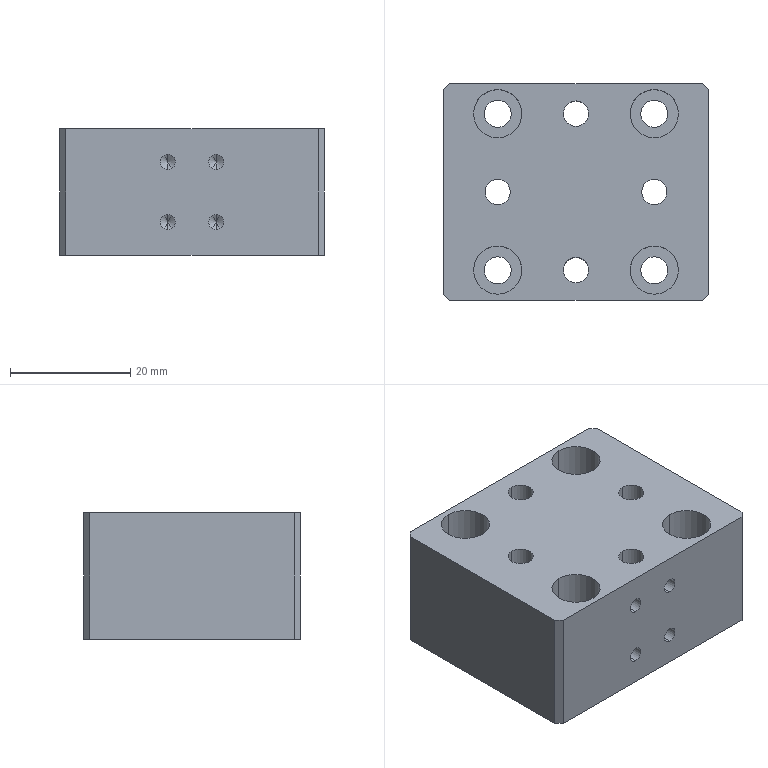NC program | NX | posted with a generic post | part box 44 x 36 x 21 mm
Whole program:
N10 G17 G21 G94 G90
(FLOOR_WALL , TOOL : D63)
N12 T01 M6
N14 G54
N16 G17 G0 G90 X-60.5 Y0. B0. C0. S6500 M3
N18 G43 Z30. H1
N20 Z3.
N22 G94 G1 Z0. F1250.
N24 X-57.5
N26 X57.5
N28 X60.5
N30 Z3.
N32 G0 Z30.
N34 M5
(DRILLING_COPY_1 , TOOL : D6A45)
N36 T07 M6
N38 G54
N40 G17 G0 G90 X-13. Y0. B0. C0. S5000 M3
N42 G43 Z30. H7
N44 G94 G81 G98 Z-2.6 F250. R3.
N46 Y13.
N48 X0.
N50 X13.
N52 Y0.
N54 Y-13.
N56 X0.
N58 X-13.
N60 G80
N62 G0 X-13. Y-13. Z30.
N64 M5
(DRILLING_COPY , TOOL : 4.2ZT)
N66 T14 M6
N68 G54
N70 G17 G0 G90 X-13. Y0. B0. C0. S2000 M3
N72 G43 Z30. H14
N74 G94 G83 G98 Z-23.762 F150. Q2. R3.
N76 X0. Y13.
N78 X13. Y0.
N80 X0. Y-13.
N82 G80
N84 G0 X0. Y-13. Z30.
N86 M5
(DRILLING_COPY_COPY_1 , TOOL : 4.5ZT)
N88 T16 M6
N90 G54
N92 G17 G0 G90 X-13. Y13. B0. C0. S2000 M3
N94 G43 Z30. H16
N96 G94 G83 G98 Z-23.852 F150. Q2. R3.
N98 X13.
N100 Y-13.
N102 X-13.
N104 G80
N106 G0 X-13. Y-13. Z30.
N108 M5
(HOLE_MILLING , TOOL : D4)
N110 T04 M6
N112 G54
N114 G17 G0 G90 X-13. Y13. B0. C0. S9500 M3
N116 G43 Z30. H4
N118 Z0.5
N120 G94 G3 X-12.01 Y12.01 R0.99 F1400.
N122 X-11.02 Y13. R0.99
N124 X-11.02 Y13. Z0. I-1.98 J0.
N126 X-11.02 Y13. Z-0.5 I-1.98 J0.
N128 X-11.02 Y13. Z-1. I-1.98 J0.
N130 X-11.02 Y13. Z-1.5 I-1.98 J0.
N132 X-11.02 Y13. Z-2. I-1.98 J0.
N134 X-11.02 Y13. Z-2.5 I-1.98 J0.
N136 X-11.02 Y13. Z-3. I-1.98 J0.
N138 X-11.02 Y13. Z-3.5 I-1.98 J0.
N140 X-11.02 Y13. Z-4. I-1.98 J0.
N142 X-11.02 Y13. Z-4.5 I-1.98 J0.
N144 X-11.02 Y13. Z-5. I-1.98 J0.
N146 X-11.02 Y13. Z-5.5 I-1.98 J0.
N148 X-11.02 Y13. Z-6. I-1.98 J0.
N150 X-11.02 Y13. Z-6.5 I-1.98 J0.
N152 X-11.02 Y13. Z-7. I-1.98 J0.
N154 X-11.02 Y13. Z-7.5 I-1.98 J0.
N156 X-11.02 Y13. Z-8. I-1.98 J0.
N158 X-11.02 Y13. Z-8.5 I-1.98 J0.
N160 X-11.02 Y13. Z-9. I-1.98 J0.
N162 X-11.02 Y13. Z-9.5 I-1.98 J0.
N164 X-11.02 Y13. Z-10. I-1.98 J0.
N166 X-11.02 Y13. Z-10.5 I-1.98 J0.
N168 X-11.02 Y13. Z-11. I-1.98 J0.
N170 X-11.02 Y13. Z-11.5 I-1.98 J0.
N172 X-11.02 Y13. Z-12. I-1.98 J0.
N174 X-11.02 Y13. Z-12.5 I-1.98 J0.
N176 X-11.02 Y13. Z-13. I-1.98 J0.
N178 X-11.02 Y13. Z-13.5 I-1.98 J0.
N180 X-11.02 Y13. Z-14. I-1.98 J0.
N182 X-11.02 Y13. Z-14.5 I-1.98 J0.
N184 X-11.02 Y13. Z-15. I-1.98 J0.
N186 X-13. Y14.98 R1.98
N188 X-11.02 Y13. R-1.98
N190 X-12.01 Y13.99 R0.99
N192 X-13. Y13. R0.99
N194 G0 Z30.
N196 X13.
N198 Z0.5
N200 G3 X13.99 Y12.01 R0.99
N202 X14.98 Y13. R0.99
N204 X14.98 Y13. Z0. I-1.98 J0.
N206 X14.98 Y13. Z-0.5 I-1.98 J0.
N208 X14.98 Y13. Z-1. I-1.98 J0.
N210 X14.98 Y13. Z-1.5 I-1.98 J0.
N212 X14.98 Y13. Z-2. I-1.98 J0.
N214 X14.98 Y13. Z-2.5 I-1.98 J0.
N216 X14.98 Y13. Z-3. I-1.98 J0.
N218 X14.98 Y13. Z-3.5 I-1.98 J0.
N220 X14.98 Y13. Z-4. I-1.98 J0.
N222 X14.98 Y13. Z-4.5 I-1.98 J0.
N224 X14.98 Y13. Z-5. I-1.98 J0.
N226 X14.98 Y13. Z-5.5 I-1.98 J0.
N228 X14.98 Y13. Z-6. I-1.98 J0.
N230 X14.98 Y13. Z-6.5 I-1.98 J0.
N232 X14.98 Y13. Z-7. I-1.98 J0.
N234 X14.98 Y13. Z-7.5 I-1.98 J0.
N236 X14.98 Y13. Z-8. I-1.98 J0.
N238 X14.98 Y13. Z-8.5 I-1.98 J0.
N240 X14.98 Y13. Z-9. I-1.98 J0.
N242 X14.98 Y13. Z-9.5 I-1.98 J0.
N244 X14.98 Y13. Z-10. I-1.98 J0.
N246 X14.98 Y13. Z-10.5 I-1.98 J0.
N248 X14.98 Y13. Z-11. I-1.98 J0.
N250 X14.98 Y13. Z-11.5 I-1.98 J0.
N252 X14.98 Y13. Z-12. I-1.98 J0.
N254 X14.98 Y13. Z-12.5 I-1.98 J0.
N256 X14.98 Y13. Z-13. I-1.98 J0.
N258 X14.98 Y13. Z-13.5 I-1.98 J0.
N260 X14.98 Y13. Z-14. I-1.98 J0.
N262 X14.98 Y13. Z-14.5 I-1.98 J0.
N264 X14.98 Y13. Z-15. I-1.98 J0.
N266 X13. Y14.98 R1.98
N268 X14.98 Y13. R-1.98
N270 X13.99 Y13.99 R0.99
N272 X13. Y13. R0.99
N274 G0 Z30.
N276 Y-13.
N278 Z0.5
N280 G3 X13.99 Y-13.99 R0.99
N282 X14.98 Y-13. R0.99
N284 X14.98 Y-13. Z0. I-1.98 J0.
N286 X14.98 Y-13. Z-0.5 I-1.98 J0.
N288 X14.98 Y-13. Z-1. I-1.98 J0.
N290 X14.98 Y-13. Z-1.5 I-1.98 J0.
N292 X14.98 Y-13. Z-2. I-1.98 J0.
N294 X14.98 Y-13. Z-2.5 I-1.98 J0.
N296 X14.98 Y-13. Z-3. I-1.98 J0.
N298 X14.98 Y-13. Z-3.5 I-1.98 J0.
N300 X14.98 Y-13. Z-4. I-1.98 J0.
N302 X14.98 Y-13. Z-4.5 I-1.98 J0.
N304 X14.98 Y-13. Z-5. I-1.98 J0.
N306 X14.98 Y-13. Z-5.5 I-1.98 J0.
N308 X14.98 Y-13. Z-6. I-1.98 J0.
N310 X14.98 Y-13. Z-6.5 I-1.98 J0.
N312 X14.98 Y-13. Z-7. I-1.98 J0.
N314 X14.98 Y-13. Z-7.5 I-1.98 J0.
N316 X14.98 Y-13. Z-8. I-1.98 J0.
N318 X14.98 Y-13. Z-8.5 I-1.98 J0.
N320 X14.98 Y-13. Z-9. I-1.98 J0.
N322 X14.98 Y-13. Z-9.5 I-1.98 J0.
N324 X14.98 Y-13. Z-10. I-1.98 J0.
N326 X14.98 Y-13. Z-10.5 I-1.98 J0.
N328 X14.98 Y-13. Z-11. I-1.98 J0.
N330 X14.98 Y-13. Z-11.5 I-1.98 J0.
N332 X14.98 Y-13. Z-12. I-1.98 J0.
N334 X14.98 Y-13. Z-12.5 I-1.98 J0.
N336 X14.98 Y-13. Z-13. I-1.98 J0.
N338 X14.98 Y-13. Z-13.5 I-1.98 J0.
N340 X14.98 Y-13. Z-14. I-1.98 J0.
N342 X14.98 Y-13. Z-14.5 I-1.98 J0.
N344 X14.98 Y-13. Z-15. I-1.98 J0.
N346 X13. Y-11.02 R1.98
N348 X14.98 Y-13. R-1.98
N350 X13.99 Y-12.01 R0.99
N352 X13. Y-13. R0.99
N354 G0 Z30.
N356 X-13.
N358 Z0.5
N360 G3 X-12.01 Y-13.99 R0.99
N362 X-11.02 Y-13. R0.99
N364 X-11.02 Y-13. Z0. I-1.98 J0.
N366 X-11.02 Y-13. Z-0.5 I-1.98 J0.
N368 X-11.02 Y-13. Z-1. I-1.98 J0.
N370 X-11.02 Y-13. Z-1.5 I-1.98 J0.
N372 X-11.02 Y-13. Z-2. I-1.98 J0.
N374 X-11.02 Y-13. Z-2.5 I-1.98 J0.
N376 X-11.02 Y-13. Z-3. I-1.98 J0.
N378 X-11.02 Y-13. Z-3.5 I-1.98 J0.
N380 X-11.02 Y-13. Z-4. I-1.98 J0.
N382 X-11.02 Y-13. Z-4.5 I-1.98 J0.
N384 X-11.02 Y-13. Z-5. I-1.98 J0.
N386 X-11.02 Y-13. Z-5.5 I-1.98 J0.
N388 X-11.02 Y-13. Z-6. I-1.98 J0.
N390 X-11.02 Y-13. Z-6.5 I-1.98 J0.
N392 X-11.02 Y-13. Z-7. I-1.98 J0.
N394 X-11.02 Y-13. Z-7.5 I-1.98 J0.
N396 X-11.02 Y-13. Z-8. I-1.98 J0.
N398 X-11.02 Y-13. Z-8.5 I-1.98 J0.
N400 X-11.02 Y-13. Z-9. I-1.98 J0.
N402 X-11.02 Y-13. Z-9.5 I-1.98 J0.
N404 X-11.02 Y-13. Z-10. I-1.98 J0.
N406 X-11.02 Y-13. Z-10.5 I-1.98 J0.
N408 X-11.02 Y-13. Z-11. I-1.98 J0.
N410 X-11.02 Y-13. Z-11.5 I-1.98 J0.
N412 X-11.02 Y-13. Z-12. I-1.98 J0.
N414 X-11.02 Y-13. Z-12.5 I-1.98 J0.
N416 X-11.02 Y-13. Z-13. I-1.98 J0.
N418 X-11.02 Y-13. Z-13.5 I-1.98 J0.
N420 X-11.02 Y-13. Z-14. I-1.98 J0.
N422 X-11.02 Y-13. Z-14.5 I-1.98 J0.
N424 X-11.02 Y-13. Z-15. I-1.98 J0.
N426 X-13. Y-11.02 R1.98
N428 X-11.02 Y-13. R-1.98
N430 X-12.01 Y-12.01 R0.99
N432 X-13. Y-13. R0.99
N434 G0 Z30.
(HOLE_MILLING_COPY , TOOL : D4)
N436 Y13.
N438 Z0.5
N440 G3 X-12. Y12. R1.
N442 X-11. Y13. R1.
N444 X-11. Y13. Z-1.5 I-2. J0.
N446 X-11. Y13. Z-3.5 I-2. J0.
N448 X-11. Y13. Z-5.5 I-2. J0.
N450 X-11. Y13. Z-7.5 I-2. J0.
N452 X-11. Y13. Z-9.5 I-2. J0.
N454 X-11. Y13. Z-11.5 I-2. J0.
N456 X-11. Y13. Z-13.5 I-2. J0.
N458 X-13. Y11. Z-15. R-2.
N460 X-11. Y13. R2.
N462 X-13. Y11. R-2.
N464 X-12. Y12. R1.
N466 X-13. Y13. R1.
N468 G0 Z30.
N470 X13.
N472 Z0.5
N474 G3 X14. Y12. R1.
N476 X15. Y13. R1.
N478 X15. Y13. Z-1.5 I-2. J0.
N480 X15. Y13. Z-3.5 I-2. J0.
N482 X15. Y13. Z-5.5 I-2. J0.
N484 X15. Y13. Z-7.5 I-2. J0.
N486 X15. Y13. Z-9.5 I-2. J0.
N488 X15. Y13. Z-11.5 I-2. J0.
N490 X15. Y13. Z-13.5 I-2. J0.
N492 X13. Y11. Z-15. R-2.
N494 X15. Y13. R2.
N496 X13. Y11. R-2.
N498 X14. Y12. R1.
N500 X13. Y13. R1.
N502 G0 Z30.
N504 Y-13.
N506 Z0.5
N508 G3 X14. Y-14. R1.
N510 X15. Y-13. R1.
N512 X15. Y-13. Z-1.5 I-2. J0.
N514 X15. Y-13. Z-3.5 I-2. J0.
N516 X15. Y-13. Z-5.5 I-2. J0.
N518 X15. Y-13. Z-7.5 I-2. J0.
N520 X15. Y-13. Z-9.5 I-2. J0.
N522 X15. Y-13. Z-11.5 I-2. J0.
N524 X15. Y-13. Z-13.5 I-2. J0.
N526 X13. Y-15. Z-15. R-2.
N528 X15. Y-13. R2.
N530 X13. Y-15. R-2.
N532 X14. Y-14. R1.
N534 X13. Y-13. R1.
N536 G0 Z30.
N538 X-13.
N540 Z0.5
N542 G3 X-12. Y-14. R1.
N544 X-11. Y-13. R1.
N546 X-11. Y-13. Z-1.5 I-2. J0.
N548 X-11. Y-13. Z-3.5 I-2. J0.
N550 X-11. Y-13. Z-5.5 I-2. J0.
N552 X-11. Y-13. Z-7.5 I-2. J0.
N554 X-11. Y-13. Z-9.5 I-2. J0.
N556 X-11. Y-13. Z-11.5 I-2. J0.
N558 X-11. Y-13. Z-13.5 I-2. J0.
N560 X-13. Y-15. Z-15. R-2.
N562 X-11. Y-13. R2.
N564 X-13. Y-15. R-2.
N566 X-12. Y-14. R1.
N568 X-13. Y-13. R1.
N570 G0 Z30.
N572 M5
(ADAPTIVE_MILLING , TOOL : D10)
N574 T10 M6
N576 G54
N578 G17 G0 G90 X-33.697 Y-0.05 B0. C0. S9500 M3
N580 G43 Z30. H10
N582 Z-20.
N584 G94 G1 Z-21. F1000.
N586 X-32.34 Y-0.58 F3000.
N588 G3 X-31.05 Y-0.05 R1.015
N590 X-30.406 Y3.11 R9.424
N592 X-30.21 Y14.606 R185.073
N594 G2 X-30.164 Y19.904 R87.231
N596 X-27.107 Y24.146 R6.172
N598 X-21.408 Y25.863 R13.799
N600 X-11.818 Y26.181 R97.285
N602 G1 X-9.818 Y26.186
N604 X-6.418 Y26.189
N606 X4.482 Y26.19
N608 X23.282
N610 X23.382 Y26.189
N612 X23.482 Y26.186
N614 G2 X27.916 Y23.446 R5.892
N616 X29.812 Y17.813 R12.753
N618 X30.178 Y8.626 R81.53
N620 G1 X30.184 Y6.926
N622 X30.188 Y4.426
N624 X30.19 Y-0.574
N626 X30.191 Y-19.274
N628 X30.19 Y-19.374
N630 X30.187 Y-19.474
N632 G2 X27.452 Y-23.911 R5.888
N634 X21.821 Y-25.812 R12.766
N636 X13.133 Y-26.175 R76.729
N638 G1 X11.633 Y-26.182
N640 X9.533 Y-26.187
N642 X6.033 Y-26.189
N644 X-6.567 Y-26.19
N646 X-23.267
N648 X-23.367
N650 G2 X-27.732 Y-23.703 R5.738
N652 X-29.742 Y-18.325 R11.924
N654 X-30.171 Y-9.843 R63.748
N656 X-30.136 Y-2.144 R153.414
N658 G3 X-29.43 Y12.529 R119.594
N660 G2 X-29.366 Y17.427 R77.262
N662 X-25.308 Y23.173 R7.786
N664 X-19.116 Y24.995 R16.033
N666 X-9.728 Y25.365 R90.974
N668 G1 X-8.228 Y25.372
N670 X-6.128 Y25.377
N672 X-2.828 Y25.38
N674 X5.672 Y25.382
N676 X20.472
N678 X20.672 Y25.38
N680 G2 X26.938 Y21.67 R7.557
N682 X28.965 Y15.341 R15.177
N684 X29.361 Y6.455 R81.33
N686 G1 X29.369 Y5.055
N688 X29.375 Y3.355
N690 X29.379 Y0.755
N692 X29.382 Y-4.045
N694 Y-16.545
N696 X29.381 Y-16.645
N698 G2 X25.691 Y-22.923 R7.563
N700 X19.466 Y-24.95 R15.025
N702 X9.781 Y-25.364 R84.712
N704 G1 X8.281 Y-25.371
N706 X6.281 Y-25.376
N708 X3.081 Y-25.38
N710 X-4.219 Y-25.382
N712 X-20.519
N714 X-20.619 Y-25.381
N716 G2 X-26.964 Y-21.629 R7.577
N718 X-28.974 Y-15.295 R15.341
N720 X-29.03 Y0.681 R86.884
N722 G3 X-28.624 Y14.672 R206.127
N724 G2 X-23.838 Y22.258 R8.821
N726 X-21.472 Y23.305 R8.031
N728 X-13.975 Y24.417 R29.802
N730 X0.523 Y24.572 R399.715
N732 G1 X9.523 Y24.573
N734 X18.223
N736 X18.423 Y24.57
N738 X18.623 Y24.566
N740 X18.823 Y24.558
N742 X18.923 Y24.553
N744 G2 X26.171 Y19.952 R8.759
N746 X27.179 Y17.851 R6.56
N748 X28.387 Y10.574 R27.305
N750 X28.571 Y-3.323 R311.808
N752 X28.533 Y-15.222 R436.293
N754 X23.946 Y-22.176 R8.77
N756 X21.851 Y-23.179 R6.583
N758 X14.774 Y-24.371 R26.639
N760 X2.077 Y-24.57 R260.792
N762 G1 X-2.323 Y-24.572
N764 X-18.123 Y-24.573
N766 X-18.323 Y-24.572
N768 X-18.623 Y-24.566
N770 X-18.823 Y-24.558
N772 X-18.923 Y-24.553
N774 G2 X-26.183 Y-19.936 R8.78
N776 X-27.18 Y-17.852 R6.64
N778 X-28.392 Y-10.475 R27.444
N780 X-28.184 Y1.215 R92.775
N782 G3 X-27.833 Y13.008 R314.175
N784 G2 X-27.154 Y16.428 R13.151
N786 X-26.418 Y19.63 R6.131
N788 X-23.821 Y22.271 R10.862
N790 G1 X-23.63 Y22.418
N792 X-23.511 Y22.486
N794 G2 X-20.466 Y23.16 R6.28
N796 X-1.882 Y23.758 R211.897
N798 G1 X1.418 Y23.762
N800 X7.518 Y23.764
N802 X16.018 Y23.765
N804 X16.318 Y23.762
N806 X16.718 Y23.755
N808 X16.918 Y23.748
N810 G2 X20.28 Y23.15 R13.765
N812 X23.511 Y22.486 R6.269
N814 X26.21 Y19.9 R10.464
N816 G3 X27.903 Y20.947 R1.
N818 G1 X27.05 Y22.756 Z-20.9
N820 X26.408 Y24.119
N822 X26.318 Y24.266
N824 X26.21 Y24.4
N826 X25.587 Y25.007
N828 G3 X24.728 Y25.465 R2.608
N830 X21.706 Y26.16 R16.644
N832 X16.12 Y26.725 R75.358
N834 G1 X14.874 Y26.774
N836 X13.627 Y26.802
N838 X-18.516 Y27.047
N840 G3 X-19.169 Y26.811 R1.032
N842 G1 X-20.522 Y25.666
N844 X-21.034 Y25.24 Z-20.933
N846 X-21.529 Y24.795 Z-20.967
N848 G3 X-21.765 Y24.184 Z-21. R1.04
N850 X-20.766 Y23.15 R1.004
N852 G1 X20.334
N854 G2 X23.63 Y22.418 R6.139
N856 X26.486 Y19.511 R10.886
N858 X27.16 Y16.466 R6.28
N860 X27.752 Y0.082 R184.971
N862 X27.728 Y-13.317 R641.242
N864 X27.15 Y-16.278 R14.406
N866 X26.486 Y-19.511 R6.27
N868 X23.9 Y-22.21 R10.464
N870 G3 X24.947 Y-23.903 R1.
N872 G1 X26.756 Y-23.05 Z-20.9
N874 X28.119 Y-22.408
N876 X28.266 Y-22.318
N878 X28.4 Y-22.21
N880 X29.007 Y-21.587
N882 G3 X29.466 Y-20.728 R2.611
N884 X30.158 Y-17.706 R16.322
N886 X30.713 Y-12.12 R79.161
N888 G1 X30.763 Y-10.874
N890 X30.794 Y-9.628
N892 X31.047 Y14.516
N894 G3 X30.81 Y15.172 R1.032
N896 G1 X29.666 Y16.523
N898 X29.239 Y17.034 Z-20.933
N900 X28.795 Y17.53 Z-20.967
N902 G3 X28.183 Y17.765 Z-21. R1.04
N904 X27.15 Y16.766 R1.004
N906 G1 Y-16.334
N908 G2 X26.418 Y-19.63 R6.139
N910 X23.511 Y-22.486 R10.886
N912 X20.466 Y-23.16 R6.28
N914 X3.882 Y-23.752 R190.383
N916 G1 X1.582 Y-23.758
N918 X-1.718 Y-23.762
N920 X-8.318 Y-23.764
N922 X-16.018 Y-23.765
N924 X-16.318 Y-23.762
N926 X-16.718 Y-23.755
N928 G2 X-20.278 Y-23.15 R13.593
N930 X-23.511 Y-22.486 R6.271
N932 X-26.21 Y-19.9 R10.464
N934 G3 X-27.903 Y-20.947 R1.
N936 G1 X-27.05 Y-22.756 Z-20.9
N938 X-26.408 Y-24.119
N940 X-26.318 Y-24.266
N942 X-26.21 Y-24.4
N944 X-25.587 Y-25.007
N946 G3 X-24.728 Y-25.465 R2.608
N948 X-21.706 Y-26.16 R16.644
N950 X-16.12 Y-26.725 R75.358
N952 G1 X-14.874 Y-26.774
N954 X-13.627 Y-26.802
N956 X18.516 Y-27.047
N958 G3 X19.169 Y-26.811 R1.032
N960 G1 X20.522 Y-25.666
N962 X21.034 Y-25.24 Z-20.933
N964 X21.529 Y-24.795 Z-20.967
N966 G3 X21.765 Y-24.184 Z-21. R1.04
N968 X20.766 Y-23.15 R1.004
N970 G1 X-20.334
N972 G2 X-23.63 Y-22.418 R6.139
N974 X-26.486 Y-19.511 R10.886
N976 X-27.156 Y-16.566 R6.158
N978 X-27.658 Y-6.481 R153.028
N980 X-27.207 Y5.41 R516.415
N982 G3 X-27.15 Y16.522 R389.897
N984 X-28.252 Y17.62 R1.1
N986 X-29.35 Y16.522 R1.1
N988 G1 Y-16.766
N990 G3 X-28.248 Y-17.864 R1.1
N992 X-27.15 Y-16.766 R1.1
N994 G1 Y7.634
N996 G3 X-28.011 Y8.633 R1.016
N998 G1 X-29.604 Y8.871
N1000 Z-18.
N1002 G0 Z30.
N1004 M5
(ZLEVEL_PROFILE_COPY_COPY_1 , TOOL : D10JING)
N1006 T11 M6
N1008 G54
N1010 G17 G0 G90 X-27.438 Y-17.827 B0. C0. S9500 M3
N1012 G43 Z30. H11
N1014 Z-18.
N1016 G94 G1 Z-21. F1200.
N1018 G3 X-27. Y-17. R1.
N1020 G1 Y17.
N1022 G2 X-25.536 Y20.536 R5.
N1024 G1 X-24.536 Y21.536
N1026 G2 X-21. Y23. R5.
N1028 G1 X21.
N1030 G2 X24.536 Y21.536 R5.
N1032 G1 X25.536 Y20.536
N1034 G2 X27. Y17. R5.
N1036 G1 Y-17.
N1038 G2 X25.536 Y-20.536 R5.
N1040 G1 X24.536 Y-21.536
N1042 G2 X21. Y-23. R5.
N1044 G1 X-21.
N1046 G2 X-24.536 Y-21.536 R5.
N1048 G1 X-25.536 Y-20.536
N1050 G2 X-27. Y-17. R5.
N1052 G3 X-27.5 Y-16.134 R1.
N1054 G1 Z-18.
N1056 G0 Z30.
N1058 M5
(ZLEVEL_PROFILE_1_COPY_1 , TOOL : D6A45)
N1060 T07 M6
N1062 G54
N1064 G17 G0 G90 X14.439 Y14.149 B0. C0. S9500 M3
N1066 G43 Z30. H7
N1068 Z0.
N1070 G94 G1 Z-1. F1000.
N1072 X13.52 Y15.741
N1074 G3 X13. Y16.041 R0.6
N1076 G1 X12.998
N1078 G3 X9.959 Y12.998 R3.041
N1080 X13. Y16.041 R-3.041
N1082 X12.48 Y15.741 R0.6
N1084 G1 X11.561 Y14.149
N1086 Z0.
N1088 G0 Z30.
N1090 X-11.561
N1092 Z0.
N1094 G1 Z-1.
N1096 X-12.48 Y15.741
N1098 G3 X-13. Y16.041 R0.6
N1100 X-16.041 Y13. R3.041
N1102 X-13. Y16.041 R-3.041
N1104 X-13.52 Y15.741 R0.6
N1106 G1 X-14.439 Y14.149
N1108 Z0.
N1110 G0 Z30.
N1112 X14.141 Y0.
N1114 Z1.
N1116 G1 Z-1.
N1118 G3 X13. Y1.141 R1.141
N1120 X14.141 Y0. R-1.141
N1122 X13.841 Y0.52 R0.6
N1124 G1 Z0.
N1126 G0 Z30.
N1128 X-14.141 Y0.
N1130 Z1.
N1132 G1 Z-1.
N1134 G3 X-13. Y-1.141 R1.141
N1136 X-14.141 Y0. R-1.141
N1138 X-13.841 Y-0.52 R0.6
N1140 G1 Z0.
N1142 G0 Z30.
N1144 X0. Y-14.141
N1146 Z1.
N1148 G1 Z-1.
N1150 X0.005
N1152 G3 X1.141 Y-12.995 R1.141
N1154 X0. Y-14.141 R-1.141
N1156 X0.52 Y-13.841 R0.6
N1158 G1 Z0.
N1160 G0 Z30.
N1162 X11.561 Y-14.149
N1164 Z0.
N1166 G1 Z-1.
N1168 X12.48 Y-15.741
N1170 G3 X13. Y-16.041 R0.6
N1172 X16.041 Y-13. R3.041
N1174 X13. Y-16.041 R-3.041
N1176 X13.52 Y-15.741 R0.6
N1178 G1 X14.439 Y-14.149
N1180 Z0.
N1182 G0 Z30.
N1184 X-14.439
N1186 Z0.
N1188 G1 Z-1.
N1190 X-13.52 Y-15.741
N1192 G3 X-13. Y-16.041 R0.6
N1194 G1 X-12.997
N1196 G3 X-9.959 Y-12.997 R3.041
N1198 X-13. Y-16.041 R-3.041
N1200 X-12.48 Y-15.741 R0.6
N1202 G1 X-11.561 Y-14.149
N1204 Z0.
N1206 G0 Z30.
N1208 X0. Y14.141
N1210 Z1.
N1212 G1 Z-1.
N1214 X-0.008
N1216 G3 X-1.141 Y12.992 R1.141
N1218 X0. Y14.141 R-1.141
N1220 X-0.52 Y13.841 R0.6
N1222 G1 Z0.
N1224 G0 Z30.
N1226 X-21.921 Y19.952
N1228 Z0.
N1230 G1 Z-1.
N1232 X-21.52 Y19.259
N1234 G3 X-21.001 Y18.959 R0.6
N1236 G1 X21.001
N1238 G2 X21.677 Y18.678 R0.957
N1240 G1 X22.678 Y17.677
N1242 G2 X22.959 Y17.001 R0.956
N1244 G1 Y-17.001
N1246 G2 X22.678 Y-17.677 R0.956
N1248 G1 X21.677 Y-18.678
N1250 G2 X21.001 Y-18.959 R0.957
N1252 G1 X-21.001
N1254 G2 X-21.677 Y-18.678 R0.957
N1256 G1 X-22.678 Y-17.677
N1258 G2 X-22.959 Y-17.001 R0.956
N1260 G1 Y17.001
N1262 G2 X-22.678 Y17.677 R0.956
N1264 G1 X-21.677 Y18.678
N1266 G2 X-21.001 Y18.959 R0.957
N1268 G3 X-20.481 Y19.259 R0.6
N1270 G1 X-19.962 Y20.159
N1272 Z0.
N1274 G0 Z30.
N1276 M5
N1278 M2